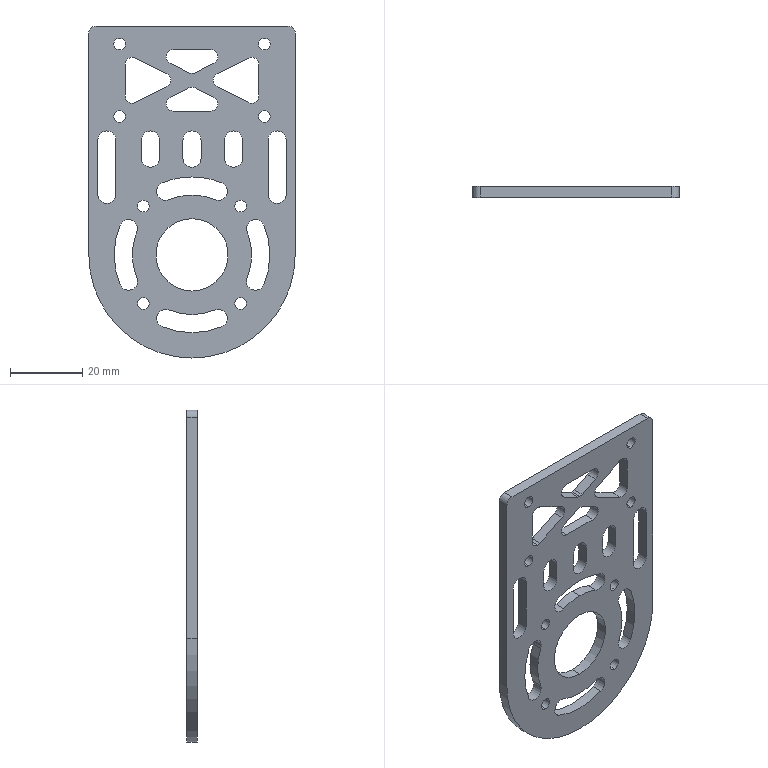Part | SolidWorks | features Extrusion 1, Fillet 1, ICE 1 | 1 solid | 101 faces | box 57 x 3 x 91.7 mm | volume 10337 mm3 | cylinder 74 | plane 27 | commonest cylinder face diameters 5 x27 4 x17 3.2 x16 33 x5 43 x5 20 x2